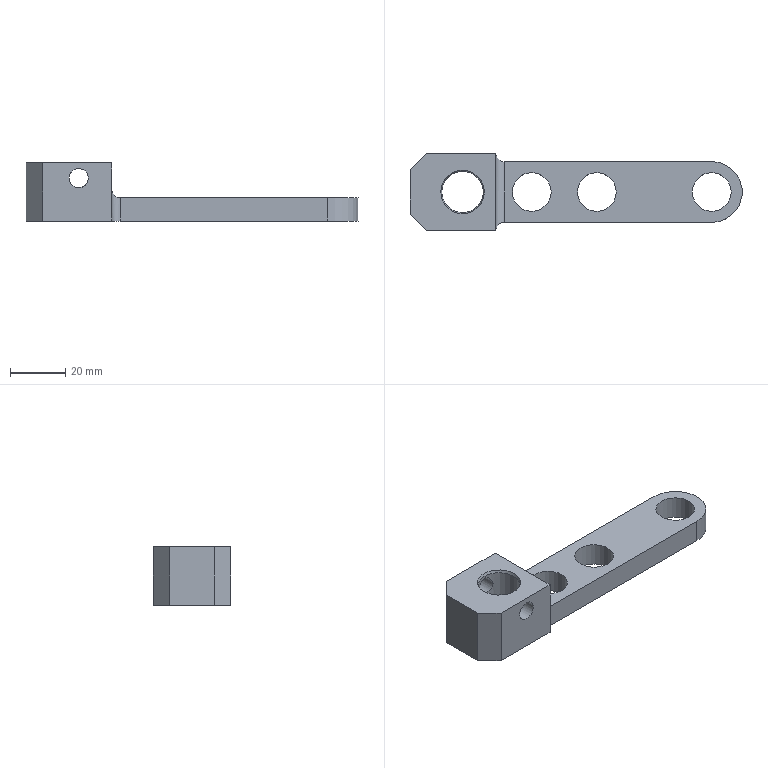NC program | NX | posted with a generic post | part box 120 x 28 x 21 mm
Lines 1 to 817 of 4754:
N10 G17 G21 G94 G90
(动态粗_COPY , TOOL : D10-30-D10-75-3T-粗)
N12 T02 M6
N14 G54
N16 G17 G0 G90 X10.538 Y8.528 B0. C0. S4500 M3
N18 G43 Z6. H2
N20 Z-11.9
N22 G94 G1 X10.513 Y8.53 Z-12.056 F2000.
N24 X10.488 Y8.531 Z-12.118
N26 X10.463 Y8.533 Z-12.163
N28 X10.438 Y8.534 Z-12.2
N30 X10.413 Y8.535 Z-12.231
N32 X10.388 Y8.537 Z-12.257
N34 X10.363 Y8.538 Z-12.28
N36 X10.338 Y8.54 Z-12.3
N38 X10.313 Y8.541 Z-12.318
N40 X10.288 Y8.543 Z-12.333
N42 X10.263 Y8.544 Z-12.347
N44 X10.238 Y8.545 Z-12.358
N46 X10.213 Y8.547 Z-12.368
N48 X10.188 Y8.548 Z-12.377
N50 X10.163 Y8.55 Z-12.384
N52 X10.138 Y8.551 Z-12.39
N54 X10.113 Y8.553 Z-12.394
N56 X10.089 Y8.554 Z-12.397
N58 X10.064 Y8.555 Z-12.399
N60 X10.039 Y8.557 Z-12.4
N62 X8.546 Y8.643
N64 G3 X7.508 Y7.879 R1.01
N66 X7.317 Y4.783 R18.753
N68 G1 X7.3 Y-0.166
N70 Y-13.665
N72 G2 X4.671 Y-18.222 R5.622
N74 X0.422 Y-19.616 R9.406
N76 X-4.852 Y-19.795 R53.755
N78 G1 X-8.512 Y-19.8
N80 X-121.12 Y-19.799
N82 G2 X-125.704 Y-17.192 R5.608
N84 X-127.105 Y-12.993 R9.323
N86 X-127.296 Y-7.224 R56.034
N88 G1 X-127.299 Y-3.624
N90 Y13.704
N92 G2 X-124.635 Y18.242 R5.634
N94 X-120.462 Y19.609 R9.412
N96 X-114.738 Y19.797 R56.511
N98 G1 X-111.138 Y19.8
N100 X1.21 Y19.798
N102 G2 X5.737 Y17.142 R5.633
N104 X7.119 Y12.868 R9.502
N106 X7.172 Y6.565 R41.659
N108 G3 X7.1 Y-5.331 R443.864
N110 G2 X7.078 Y-12.81 R298.984
N112 X3.379 Y-18.221 R6.758
N114 X-1.172 Y-19.434 R11.824
N116 X-7.693 Y-19.597 R82.236
N118 G1 X-10.783 Y-19.599
N120 X-119.765
N122 G2 X-125.66 Y-15.986 R6.715
N124 X-126.925 Y-11.406 R11.612
N126 X-127.096 Y-5.396 R71.864
N128 G1 X-127.099 Y-1.766
N130 X-127.098 Y12.354
N132 G2 X-123.451 Y18.179 R6.723
N134 X-118.932 Y19.423 R11.634
N136 X-112.996 Y19.596 R69.91
N138 G1 X-109.366 Y19.599
N140 X-0.146 Y19.598
N142 G2 X5.679 Y15.951 R6.723
N144 X6.929 Y11.364 R11.709
N146 X6.968 Y6.558 R40.739
N148 G3 X6.9 Y-10.921 R915.071
N150 G2 X2.447 Y-18.104 R7.514
N152 X-2.314 Y-19.238 R13.605
N154 X-9.6 Y-19.397 R102.013
N156 G1 X-12.48 Y-19.399
N158 X-118.475
N160 G2 X-125.623 Y-14.9 R7.517
N162 X-126.749 Y-10.045 R13.888
N164 X-126.898 Y-2.278 R116.141
N166 G1 X-126.899 Y10.959
N168 G2 X-122.384 Y18.131 R7.522
N170 X-117.541 Y19.25 R13.919
N172 X-109.789 Y19.398 R115.93
N174 G1 X-1.526 Y19.399
N176 G2 X5.592 Y14.965 R7.506
N178 X6.734 Y9.828 R13.309
N180 X6.719 Y3.366 R144.577
N182 G1 X6.69 Y-10.546
N184 G2 X1.74 Y-17.922 R8.049
N186 X-3.287 Y-19.042 R15.039
N188 G3 X-6.001 Y-19.2 R88.888
N190 G1 X-32.286
N192 X-117.501 Y-19.199
N194 G2 X-122.346 Y-17.925 R8.557
N196 X-125.874 Y-13.031 R8.81
N198 X-126.615 Y-7.985 R19.932
N200 X-126.699 Y0.849 R258.101
N202 X-126.678 Y10.808 R535.414
N204 X-121.799 Y17.892 R8.025
N206 X-116.852 Y19.032 R14.764
N208 X-109.085 Y19.198 R108.819
N210 G1 X-106.61 Y19.199
N212 X-30.999 Y19.2
N214 X-3.999 Y19.199
N216 G2 X-0.795 Y19.09 R23.657
N218 X5.374 Y14.337 R8.002
N220 X6.478 Y9.341 R13.791
N222 X6.539 Y6.702 R110.831
N224 X6.478 Y-10.019 R924.614
N226 X1.199 Y-17.694 R8.493
N228 X-3.935 Y-18.828 R15.836
N230 G3 X-4.987 Y-19.1 R5.087
N232 G1 X-5.495 Y-19.15
N234 G3 X-4.159 Y-18.849 R4.499
N236 X-0.89 Y-18.218 R61.535
N238 X4.035 Y-15.414 R9.864
N240 X6.241 Y-10.163 R8.958
N242 X6.417 Y-4.084 R71.286
N244 X6.384 Y8.466 R628.675
N246 X5.486 Y13.538 R15.499
N248 X-1.451 Y18.9 R8.213
N250 X-4.909 Y19.083 R39.059
N252 G1 X-4.953 Y19.091
N254 G2 X-5.655 Y19.749 R1.001
N256 G1 X-6.115 Y21.688 Z-12.3
N258 X-6.221 Y22.12 F15000.
N260 X-6.309 Y22.556
N262 G2 X-4.953 Y23.575 R1.
N264 X-4.243 Y22.892 R1.061
N266 X-4.845 Y21.663 R1.
N268 G1 X-4.977 Y21.613
N270 X-6.311 Y21.105 Z-12.372 F2000.
N272 G3 X-6.736 Y20.745 Z-12.4 R1.007
N274 X-5.999 Y19.2 R1.
N276 G2 X-4.21 Y18.966 R20.925
N278 X-0.76 Y18.495 R23.84
N280 X5.245 Y12.996 R8.609
N282 X6.15 Y7.892 R16.45
N284 X6.219 Y0.033 R239.909
N286 X6.115 Y-8.824 R183.204
N288 X4.883 Y-13.497 R10.616
N290 X-0.132 Y-17.601 R9.314
N292 X-3.382 Y-18.481 R27.849
N294 X-4.169 Y-18.852 R5.534
N296 G3 X-3.343 Y-18.458 R5.409
N298 X-0.477 Y-17.559 R99.779
N300 X4.494 Y-13.625 R9.518
N302 X5.925 Y-8.897 R10.992
N304 X6.098 Y-2.152 R77.601
N306 X6.076 Y6.471 R397.958
N308 X5.516 Y11.514 R22.957
N310 X2.216 Y16.758 R9.331
N312 X-2.325 Y18.573 R9.963
N314 G1 X-4.138 Y18.843
N316 X-4.899 Y19.074
N318 G3 X-1.738 Y18.244 R39.019
N320 G2 X5.042 Y11.819 R9.338
N322 X5.833 Y6.659 R19.711
N324 X5.882 Y-5.823 R379.658
N326 X5.414 Y-10.411 R23.249
N328 X2.946 Y-14.93 R9.333
N330 G1 X0.662 Y-17.214
N332 G3 X0.398 Y-17.632 R1.364
N334 G1 X-0.474 Y-19.425 Z-12.3
N336 X-0.877 Y-20.254 F15000.
N338 G3 X-0.498 Y-21.545 R1.
N340 G1 X-0.325 Y-21.652
N342 X-0.157 Y-21.767
N344 G2 X-1.625 Y-23.1 R-1.
N346 G1 X-3.007 Y-21.106
N348 X-3.428 Y-20.503 Z-12.337 F2000.
N350 X-3.841 Y-19.894 Z-12.374
N352 G2 X-3.982 Y-19.399 Z-12.4 R1.006
N354 X-3.453 Y-18.506 R1.001
N356 X-1.328 Y-17.721 R17.488
N358 G3 X2.166 Y-15.45 R10.608
N360 X5.455 Y-9.118 R10.513
N362 X5.772 Y-3.762 R35.277
N364 G1 X5.776 Y5.708
N366 G3 X5.219 Y10.523 R28.532
N368 X2.161 Y15.934 R10.113
N370 X-2.26 Y18.187 R10.905
N372 G1 X-3.586 Y18.577
N374 X-4.009 Y18.803
N376 G3 X-1.79 Y17.856 R13.22
N378 G2 X3.157 Y14.241 R10.391
N380 X5.216 Y8.889 R12.348
N382 X5.566 Y3.386 R34.911
N384 G1 X5.576 Y-5.364
N386 G2 X4.966 Y-10.108 R22.895
N388 X-1.622 Y-17.474 R11.081
N390 G3 X-2.686 Y-17.975 R8.519
N392 G2 X-3.337 Y-18.444 R2.537
N394 G3 X-2.551 Y-17.876 R4.482
N396 X-0.072 Y-16.514 R63.751
N398 X4.792 Y-10.014 R11.367
N400 X5.256 Y-7.797 R7.281
N402 X5.455 Y-2.389 R48.803
N404 G1 X5.453 Y5.731
N406 X5.083 Y9.117
N408 G3 X3.251 Y13.723 R13.39
N410 X2.079 Y15.16 R11.052
N412 G1 X0.283 Y16.956
N414 G2 X0.031 Y17.38 R1.021
N416 X1.124 Y18.654 Z-12.3 R1.002
N418 G1 X1.269 Y18.622 F15000.
N420 X1.408 Y18.571
N422 X4.478 Y17.157
N424 X4.63 Y17.068
N426 X4.767 Y16.956
N428 X6.388 Y15.335
N430 G2 X7.344 Y13.237 R3.292
N432 G1 X7.43 Y12.01
N434 G2 X7.238 Y11.348 R1.005
N436 G1 X7.05 Y11.093
N438 X5.87 Y9.488 Z-12.4 F2000.
N440 X5.577 Y9.096
N442 X5.299 Y8.693
N444 G3 X5.188 Y8.127 R1.011
N446 G2 X5.253 Y-5.397 R549.731
N448 G3 X5.2 Y-8.001 R25.182
N450 G1 X5.1 Y-9.016
N452 X5.2 Y-8.001
N454 Y8.
N456 G3 X4.805 Y9.989 R6.055
N458 X2.673 Y14.158 R13.609
N460 X-2.022 Y17.747 R10.723
N462 G2 X-2.917 Y18.166 R11.664
N464 X-3.311 Y19.015 R1.001
N466 X-3.166 Y19.519 Z-12.374 R1.504
N468 G1 X-2.616 Y20.877 Z-12.3
N470 X-2.284 Y21.694 F15000.
N472 G2 X-0.675 Y22.049 R1.
N474 G1 X-0.415 Y21.809
N476 X-0.166 Y21.558
N478 G2 X-1.164 Y19.962 R1.
N480 G1 X-2.789 Y20.363 Z-12.384 F2000.
N482 X-2.947 Y20.379 Z-12.392
N484 X-3.106 Y20.372 Z-12.4
N486 G3 X-3.441 Y18.5 R1.
N488 G2 X-2.679 Y17.994 R4.582
N490 X-0.143 Y16.462 R31.336
N492 X3.992 Y11.3 R12.947
N494 G1 X4.324 Y10.888
N496 X4.805 Y9.989
N498 X4.324 Y10.888
N500 G2 X3.286 Y12.426 R9.707
N502 G3 X-1.647 Y17.218 R13.806
N504 G2 X-2.856 Y18.114 R6.817
N506 G3 X-0.329 Y16.083 R47.298
N508 G2 X3.085 Y12.269 R17.62
N510 X4.001 Y11.282 R8.895
N512 G3 X2.855 Y12.519 R18.595
N514 X-1.364 Y16.718 R23.285
N516 G1 X-2.181 Y17.535
N518 X3.037 Y12.317
N520 G3 X4.059 Y12.074 R1.001
N522 G1 X4.521 Y12.288 Z-12.374
N524 X4.975 Y12.516 Z-12.349
N526 X5.85 Y12.948 Z-12.3
N528 X6.224 Y13.12 F15000.
N530 G2 X7.521 Y12.317 R1.
N532 G1 X7.78 Y10.595
N534 X8.023 Y8.871
N536 G2 X8.324 Y4.909 R41.634
N538 G1 X8.675 Y-7.772
N540 G2 X7.962 Y-8.757 R1.
N542 G1 X7.636 Y-8.855
N544 X5.727 Y-9.425 Z-12.4 F2000.
N546 X5.264 Y-9.573
N548 G3 X4.792 Y-10.014 R1.007
N550 G2 X3.206 Y-12.877 R26.269
N552 X1.795 Y-14.584 R13.407
N554 X0.165 Y-16.183 R33.637
N556 G3 X-2.035 Y-17.397 R184.505
N558 G2 X-2.66 Y-17.953 R17.962
N560 G1 X-1.894 Y-17.28
N562 G3 X1.034 Y-15.102 R17.88
N564 X3.9 Y-11.405 R14.788
N566 X4.641 Y-10.295 R3.607
N568 G2 X3.9 Y-11.405 R3.607
N570 X1.494 Y-14.278 R38.395
N572 X-1.136 Y-16.489 R19.494
N574 G1 X-2.069 Y-17.423
N576 G2 X0.512 Y-15.025 R38.919
N578 G3 X2.884 Y-12.47 R20.143
N580 G1 X3.676 Y-11.677
N582 X-1.051 Y-16.405
N584 G3 X-1.247 Y-17.553 R1.028
N586 G1 X-0.548 Y-19.419 Z-12.3
N588 G2 X-0.417 Y-19.882 R1.544 F15000.
N590 X-1.051 Y-20.889 R1.
N592 G1 X-3.171 Y-21.707
N594 X-3.712 Y-21.886
N596 X-4.262 Y-22.035
N598 G2 X-5.183 Y-22.138 R4.839
N600 G1 X-27.83 Y-22.371
N602 G2 X-28.662 Y-21.941 R1.001
N604 G1 X-28.826 Y-21.704
N606 X-29.963 Y-20.067 Z-12.4 F2000.
N608 X-30.154 Y-19.785
N610 X-30.36 Y-19.512
N612 G3 X-31.001 Y-19.2 R1.005
N614 X-36.128 Y-19.005 R47.114
N616 G1 X-39.411 Y-19.
N618 X-116.376 Y-18.999
N620 G2 X-120.417 Y-18.405 R10.948
N622 X-125.31 Y-13.419 R8.626
N624 X-126.355 Y-8.218 R16.886
N626 X-126.497 Y-0.271 R134.652
N628 X-126.477 Y9.984 R692.384
N630 X-121.233 Y17.677 R8.488
N632 X-116.102 Y18.826 R15.741
N634 X-108.921 Y18.996 R101.92
N636 G1 X-105.996 Y18.999
N638 X-32.471
N640 X-32.248 Y19.029
N642 G3 X-31.523 Y19.872 R1.001
N644 X-31.815 Y20.713 Z-12.354 R1.047
N646 G1 X-32.508 Y21.532 Z-12.3
N648 X-32.708 Y21.765 F15000.
N650 X-32.896 Y22.008
N652 G2 X-32.248 Y23.513 R1.
N654 X-31.019 Y22.895 R1.017
N656 G1 X-30.588 Y21.714
N658 X-30.139 Y20.467 Z-12.367 F2000.
N660 G2 X-30.174 Y19.814 Z-12.4 R1.001
N662 X-31.001 Y19.2 R1.001
N664 G3 X-32.503 Y18.98 R7.645
N666 G2 X-37.235 Y18.879 R58.27
N668 G1 X-105.101
N670 G3 X-114.945 Y18.769 R223.
N672 X-120.178 Y17.885 R18.893
N674 X-125.26 Y13.641 R8.822
N676 X-126.311 Y9.224 R10.712
N678 X-126.378 Y0.735 R217.59
N680 X-126.243 Y-7.888 R155.516
N682 X-125.246 Y-13.052 R17.247
N684 X-117.982 Y-18.7 R8.632
N686 X-112.933 Y-18.877 R44.096
N688 G1 X-110.458 Y-18.879
N690 X-38.673 Y-18.88
N692 G2 X-32.423 Y-18.983 R96.355
N694 G1 X-31.928 Y-19.116
N696 G3 X-34.626 Y-18.74 R9.534
N698 X-41.736 Y-18.68 R280.612
N700 G1 X-111.471 Y-18.679
N702 G2 X-117.047 Y-18.549 R65.812
N704 X-122.611 Y-16.199 R9.255
N706 X-125.511 Y-10.962 R10.343
N708 X-126.116 Y-5.515 R26.74
N710 X-126.123 Y8.494 R342.264
N712 X-125.141 Y12.991 R11.374
N714 X-119.957 Y17.554 R9.129
N716 X-114.608 Y18.544 R18.512
N718 X-105.325 Y18.678 R175.862
N720 G1 X-39.476
N722 G3 X-33.186 Y18.761 R107.31
N724 G1 X-32.982 Y18.807
N726 G3 X-32.463 Y19.534 R1.002
N728 G1 X-32.454 Y19.791 Z-12.387
N730 X-32.471 Y20.048 Z-12.374
N732 X-32.565 Y21.523 Z-12.3
N734 X-32.617 Y22.352 F15000.
N736 G3 X-34.142 Y23.138 R1.
N738 G1 X-34.396 Y22.983
N740 X-34.641 Y22.816
N742 G3 X-34.074 Y21.056 R1.
N744 G1 X-32.445 Y20.967 Z-12.382 F2000.
N746 X-32.269 Y20.929 Z-12.391
N748 X-32.102 Y20.861 Z-12.4
N750 G2 X-32.28 Y19.019 R1.
N752 X-34.916 Y18.6 R7.682
N754 X-40.081 Y18.558 R547.93
N756 G1 X-105.686
N758 G3 X-114.549 Y18.415 R155.99
N760 X-119.818 Y17.405 R17.982
N762 X-125.754 Y10.111 R9.141
N764 X-126.049 Y5.356 R30.278
N766 X-125.96 Y-6.238 R287.079
N768 X-125.153 Y-11.608 R21.292
N770 X-121.272 Y-16.896 R9.444
N772 X-116.344 Y-18.419 R10.827
N774 X-110.017 Y-18.559 R80.121
N776 G1 X-42.315 Y-18.56
N778 G2 X-34.139 Y-18.659 R162.972
N780 X-32.943 Y-18.815 R6.107
N782 X-33.623 Y-20.695 R1.
N784 G1 X-33.808 Y-20.635
N786 X-34.701 Y-20.339 Z-12.353
N788 X-35.599 Y-20.057 Z-12.306
N790 X-35.709 Y-20.04 Z-12.3
N792 G3 X-36.113 Y-21.986 R1. F15000.
N794 G1 X-35.838 Y-22.079
N796 X-35.559 Y-22.156
N798 G3 X-34.96 Y-22.069 R1.009
N800 G1 X-33.403 Y-21.314
N802 X-32.306 Y-20.777 Z-12.361 F2000.
N804 G3 X-31.841 Y-20.187 Z-12.4 R1.
N806 X-32.537 Y-18.948 R1.
N808 G1 X-33.361 Y-18.678
N810 G3 X-37.088 Y-18.391 R21.163
N812 G1 X-43.236 Y-18.36
N814 X-109.496 Y-18.359
N816 G2 X-115.898 Y-18.22 R81.598
N818 X-120.892 Y-16.667 R10.913
N820 X-124.87 Y-11.312 R9.799
N822 X-125.741 Y-5.893 R21.049
N824 X-125.786 Y7.455 R215.609
N826 X-124.859 Y12.078 R13.328
N828 X-119.309 Y17.195 R9.445
N830 X-113.843 Y18.215 R19.034
N832 X-105.82 Y18.357 R144.795
N834 G1 X-102.85 Y18.359
N836 X-39.78
N838 G3 X-34.168 Y18.472 R74.504
N840 X-33.288 Y18.644 R3.293
N842 X-32.849 Y19.108 R1.007
N844 G1 X-32.519 Y19.824
N846 X-31.684 Y21.634 Z-12.3
N848 X-31.558 Y21.908 F15000.
N850 X-31.423 Y22.178
N852 G2 X-31.046 Y22.528 R1.017
N854 G1 X-30.823 Y22.647
N856 X-30.594 Y22.754
N858 G2 X-29.272 Y21.705 R1.
N860 X-29.79 Y20.925 Z-12.349 R1.041 F2000.
N862 G1 X-30.639 Y20.36 Z-12.4
N864 X-32.891 Y18.86
N866 G2 X-34.5 Y18.378 R3.258
N868 X-40.236 Y18.24 R68.313
N870 G1 X-42.211 Y18.238
N872 X-104.826
N874 G3 X-113.703 Y18.091 R157.127
N876 X-119.109 Y17.073 R18.827
N878 X-125.336 Y9.675 R9.575
N880 X-125.722 Y4.642 R27.891
N882 X-125.61 Y-5.886 R193.965
N884 X-124.667 Y-11.353 R19.978
N886 X-117.196 Y-17.832 R9.588
N888 X-112.148 Y-18.223 R27.745
N890 G1 X-107.258 Y-18.239
N892 X-42.468 Y-18.24
N894 G2 X-35.012 Y-18.367 R120.469
N896 X-33.306 Y-18.638 R7.99
N898 G1 X-32.982 Y-18.794
N900 G3 X-35.053 Y-18.237 R5.187
N902 X-40.824 Y-18.046 R62.867
N904 G1 X-44.826 Y-18.04
N906 X-108.081 Y-18.039
N908 G2 X-114.887 Y-17.896 R91.661
N910 X-119.927 Y-16.506 R12.305
N912 X-124.445 Y-10.905 R9.972
N914 X-125.399 Y-5.409 R20.561
N916 X-125.437 Y6.827 R147.617
N918 X-124.361 Y11.721 R13.762
N920 X-118.584 Y16.882 R9.838
N922 X-113.157 Y17.883 R19.706
N924 X-103.89 Y18.038 R161.28
N926 G1 X-43.196
N928 G3 X-35.45 Y18.131 R154.121
N930 X-33.754 Y18.397 R5.986
N932 G1 X-33.317 Y18.629
N934 G2 X-35.206 Y18.076 R4.016
N936 X-40.944 Y17.92 R65.872
N938 G1 X-42.917 Y17.918
N940 X-103.576
N942 G3 X-112.769 Y17.776 R173.328
N944 X-118.276 Y16.801 R20.239
N946 X-124.924 Y9.264 R9.955
N948 X-125.391 Y4.149 R25.916
N950 X-125.253 Y-5.613 R136.872
N952 X-124.181 Y-11.099 R18.919
N954 X-116.744 Y-17.43 R9.942
N956 X-111.598 Y-17.894 R26.267
N958 G1 X-105.868 Y-17.919
N960 X-43.429 Y-17.92
N962 G2 X-35.832 Y-18.064 R116.313
N964 X-33.737 Y-18.424 R7.724
N966 G1 X-33.711 Y-18.438
N968 G2 X-34.143 Y-20.298 R1.
N970 X-34.691 Y-20.201 Z-12.372 R1.417
N972 G1 X-36.061 Y-19.783 Z-12.3
N974 G3 X-37.431 Y-20.632 R1.011 F15000.
N976 X-36.881 Y-21.609 R1.001
N978 G1 X-36.676 Y-21.711
N980 X-36.466 Y-21.805
N982 G3 X-35.637 Y-21.713 R1.002
N984 G1 X-34.339 Y-20.934
N986 X-33.289 Y-20.298 Z-12.362 F2000.
N988 G3 X-32.88 Y-19.674 Z-12.4 R1.001
N990 X-33.428 Y-18.579 R1.
N992 X-35.536 Y-17.962 R5.08
N994 X-41.328 Y-17.729 R54.775
N996 G1 X-46.056 Y-17.72
N998 X-106.746 Y-17.719
N1000 G2 X-113.883 Y-17.581 R105.451
N1002 X-119.034 Y-16.302 R13.708
N1004 X-124.076 Y-10.366 R10.228
N1006 X-125.074 Y-4.666 R21.056
N1008 X-125.09 Y6.249 R109.89
N1010 X-123.907 Y11.318 R14.116
N1012 X-117.944 Y16.548 R10.184
N1014 X-112.308 Y17.565 R20.611
N1016 X-103.49 Y17.717 R158.554
N1018 G1 X-100.52 Y17.718
N1020 X-42.555 Y17.719
N1022 G3 X-35.85 Y17.849 R96.535
N1024 X-34.08 Y18.186 R5.686
N1026 G1 X-34.003 Y18.233
N1028 G3 X-33.57 Y18.958 R1.002
N1030 G1 X-33.533 Y19.32
N1032 X-33.329 Y21.302 Z-12.3
N1034 X-33.297 Y21.644 F15000.
N1036 X-33.248 Y21.984
N1038 G2 X-32.843 Y22.564 R1.005
N1040 G1 X-32.506 Y22.781
N1042 G2 X-31.086 Y21.699 R1.
N1044 X-31.365 Y21.165 Z-12.331 R1.099 F2000.
N1046 G1 X-32.251 Y20.105 Z-12.4
N1048 X-33.495 Y18.618
N1050 G2 X-35.2 Y17.858 R2.823
N1052 X-39.856 Y17.611 R34.191
N1054 G1 X-44.401 Y17.598
N1056 X-102.236
N1058 G3 X-111.954 Y17.456 R189.211
N1060 X-117.612 Y16.478 R21.173
N1062 X-124.558 Y8.702 R10.317
N1064 X-125.063 Y3.44 R26.106
N1066 X-124.867 Y-5.629 R95.029
N1068 X-123.566 Y-11.152 R17.228
N1070 X-116.359 Y-17.022 R10.232
N1072 X-111.222 Y-17.561 R24.665
N1074 X-104.142 Y-17.599 R603.963
N1076 G1 X-44.928 Y-17.6
N1078 G2 X-36.713 Y-17.747 R131.63
N1080 X-34.011 Y-18.236 R9.341
N1082 G1 X-33.88 Y-18.309
N1084 G2 X-34.182 Y-20.089 R1.
N1086 X-34.802 Y-20.07 Z-12.368 R1.093
N1088 G1 X-36.122 Y-19.726 Z-12.3
N1090 G3 X-37.368 Y-20.243 R1.02 F15000.
N1092 X-37.051 Y-21.48 R1.
N1094 X-36.606 Y-21.752 R1.774
N1096 X-35.659 Y-21.599 R1.001
N1098 G1 X-34.627 Y-20.797
N1100 X-34.112 Y-20.401 Z-12.333 F2000.
N1102 X-33.605 Y-19.996 Z-12.365
N1104 G3 X-33.285 Y-19.397 Z-12.4 R1.001
N1106 X-33.688 Y-18.448 R1.001
N1108 X-35.346 Y-17.788 R3.523
N1110 X-40.06 Y-17.437 R30.027
N1112 X-47.271 Y-17.4 R612.258
N1114 G1 X-105.501 Y-17.399
N1116 G2 X-113.118 Y-17.253 R112.063
N1118 X-118.368 Y-15.992 R14.599
N1120 X-123.685 Y-9.918 R10.476
N1122 X-124.74 Y-4.107 R21.083
N1124 X-124.728 Y5.891 R81.568
N1126 X-123.321 Y11.208 R13.86
N1128 X-117.346 Y16.211 R10.525
N1130 X-111.666 Y17.236 R21.112
N1132 X-102.774 Y17.396 R155.096
N1134 G1 X-99.519 Y17.398
N1136 X-43.381 Y17.399
N1138 G3 X-36.511 Y17.54 R96.911
N1140 X-34.328 Y17.982 R6.773
N1142 G1 X-33.971 Y18.255
N1144 G2 X-35.312 Y17.638 R2.51
N1146 X-39.516 Y17.309 R24.209
N1148 G1 X-46.111 Y17.278
N1150 X-101.506 Y17.277
N1152 G3 X-111.179 Y17.135 R191.785
N1154 X-116.932 Y16.169 R22.182
N1156 X-124.179 Y8.239 R10.628
N1158 X-124.731 Y2.878 R25.583
N1160 X-124.483 Y-5.514 R71.59
N1162 X-122.956 Y-11.145 R16.23
N1164 X-115.897 Y-16.641 R10.524
N1166 X-110.421 Y-17.238 R25.19
N1168 X-102.936 Y-17.279 R612.727
N1170 G1 X-45.964 Y-17.28
N1172 G2 X-37.495 Y-17.43 R139.709
N1174 X-34.445 Y-17.962 R11.219
N1176 X-33.945 Y-18.262 R2.394
N1178 G3 X-35.72 Y-17.521 R3.826
N1180 X-40.47 Y-17.128 R28.676
N1182 X-48.351 Y-17.08 R618.379
N1184 G1 X-104.371 Y-17.079
N1186 G2 X-112.198 Y-16.941 R126.511
N1188 X-117.576 Y-15.752 R15.896
N1190 X-123.344 Y-9.357 R10.739
N1192 X-124.408 Y-3.533 R21.42
N1194 X-124.36 Y5.579 R62.896
N1196 X-122.764 Y11.039 R13.684
N1198 X-116.723 Y15.891 R10.856
N1200 X-110.905 Y16.917 R21.985
N1202 X-101.278 Y17.077 R173.638
N1204 G1 X-46.451 Y17.078
N1206 G3 X-37.77 Y17.184 R181.979
N1208 X-34.851 Y17.642 R11.258
N1210 X-34.23 Y18.044 R1.853
N1212 G2 X-35.753 Y17.347 R2.865
N1214 X-40.223 Y16.991 R25.69
N1216 G1 X-46.606 Y16.958
N1218 X-100.641 Y16.957
N1220 G3 X-110.569 Y16.807 R191.107
N1222 X-116.38 Y15.826 R22.63
N1224 X-122.78 Y10.539 R10.889
N1226 X-124.252 Y5.037 R14.72
N1228 X-124.076 Y-5.521 R55.893
N1230 X-122.278 Y-11.222 R15.247
N1232 X-115.389 Y-16.281 R10.82
N1234 X-109.781 Y-16.912 R25.523
N1236 X-101.691 Y-16.96 R574.396
N1238 G1 X-47.133
N1240 G2 X-38.311 Y-17.107 R155.983
N1242 X-34.901 Y-17.67 R13.107
N1244 X-34.435 Y-17.903 R2.799
N1246 X-35.535 Y-19.547 R1.
N1248 G1 X-36.04 Y-19.238 Z-12.37
N1250 X-36.536 Y-18.915 Z-12.341
N1252 X-37.218 Y-18.479 Z-12.3
N1254 G3 X-38.318 Y-20.145 R1. F15000.
N1256 X-37.903 Y-20.403 R1.531
N1258 X-37.332 Y-20.437 R1.011
N1260 G1 X-35.741 Y-20.066
N1262 X-34.565 Y-19.786 Z-12.361 F2000.
N1264 G3 X-33.976 Y-19.301 Z-12.4 R1.
N1266 X-34.273 Y-18.024 R1.
N1268 X-35.957 Y-17.277 R3.644
N1270 X-40.497 Y-16.83 R25.169
N1272 X-49.536 Y-16.76 R384.859
N1274 G1 X-103.321 Y-16.759
N1276 G2 X-111.478 Y-16.617 R133.57
N1278 X-116.883 Y-15.471 R16.814
N1280 X-122.997 Y-8.832 R10.991
N1282 X-124.082 Y-2.859 R21.892
N1284 X-123.966 Y5.455 R48.744
N1286 X-122.058 Y11.106 R13.211
N1288 X-115.936 Y15.633 R11.268
N1290 X-109.927 Y16.613 R23.776
N1292 X-100.239 Y16.757 R196.493
N1294 G1 X-47.726 Y16.758
N1296 G3 X-38.469 Y16.865 R201.933
N1298 X-35.247 Y17.356 R12.721
N1300 X-34.717 Y17.636 R1.701
N1302 X-34.419 Y18.195 R1.008
N1304 G1 X-34.259 Y19.144
N1306 X-33.928 Y21.109 Z-12.3
N1308 X-33.85 Y21.515 F15000.
N1310 G2 X-33.557 Y21.967 R1.014
N1312 X-33.123 Y22.285 R1.671
N1314 X-31.761 Y21.644 R1.
N1316 X-32.035 Y20.636 Z-12.355 R1.036 F2000.
N1318 G1 X-32.625 Y19.961 Z-12.4
N1320 X-34.481 Y17.844
N1322 G2 X-36.369 Y17.015 R3.597
N1324 X-41.257 Y16.666 R30.754
N1326 G1 X-48.106 Y16.638
N1328 X-99.816 Y16.637
N1330 G3 X-109.908 Y16.483 R193.672
N1332 X-115.866 Y15.477 R23.15
N1334 X-122.368 Y10.142 R11.142
N1336 X-123.902 Y4.566 R14.854
N1338 X-123.655 Y-5.535 R45.273
N1340 X-121.565 Y-11.305 R14.488
N1342 X-114.79 Y-15.95 R11.145
N1344 X-109.197 Y-16.586 R26.116
N1346 X-100.487 Y-16.64 R479.165
N1348 G1 X-48.677
N1350 G2 X-39.154 Y-16.779 R184.214
N1352 X-35.399 Y-17.355 R15.401
N1354 X-34.562 Y-17.773 R2.755
N1356 X-35.536 Y-19.453 R1.
N1358 G1 X-35.75 Y-19.361 Z-12.388
N1360 X-35.949 Y-19.24 Z-12.377
N1362 X-37.247 Y-18.438 Z-12.3
N1364 G3 X-38.445 Y-20.015 R1. F15000.
N1366 X-37.962 Y-20.38 R1.353
N1368 X-37.277 Y-20.395 R1.005
N1370 G1 X-35.923 Y-19.933
N1372 X-34.754 Y-19.53 Z-12.362 F2000.
N1374 G3 X-34.226 Y-19.015 Z-12.4 R1.001
N1376 X-34.427 Y-17.909 R1.001
N1378 X-35.815 Y-17.134 R2.81
N1380 X-39.979 Y-16.562 R18.389
N1382 X-50.676 Y-16.44 R246.684
N1384 G1 X-102.471 Y-16.439
N1386 G2 X-110.779 Y-16.295 R137.644
N1388 X-116.334 Y-15.137 R17.511
N1390 X-122.644 Y-8.343 R11.222
N1392 X-123.746 Y-2.328 R21.969
N1394 X-123.554 Y5.397 R38.79
N1396 X-121.201 Y11.335 R12.723
N1398 X-115.119 Y15.384 R11.761
N1400 X-109.023 Y16.304 R25.666
N1402 X-99.605 Y16.437 R210.529
N1404 G1 X-97.04 Y16.438
N1406 X-46.814
N1408 G3 X-38.633 Y16.577 R138.384
N1410 X-35.438 Y17.145 R11.267
N1412 X-34.807 Y17.518 R1.89
N1414 X-34.566 Y17.99 R1.015
N1416 G1 X-34.324 Y19.161
N1418 X-33.921 Y21.113 Z-12.3
N1420 X-33.827 Y21.528 F15000.
N1422 X-33.751 Y21.696
N1424 X-33.647 Y21.849
N1426 G2 X-33.281 Y22.22 R1.734
N1428 X-31.765 Y21.641 R1.
N1430 X-32.043 Y20.653 Z-12.354 R1.032 F2000.
N1432 G1 X-32.651 Y19.966 Z-12.4
N1434 X-34.638 Y17.719
N1436 G2 X-35.836 Y16.955 R2.147
N1438 X-39.506 Y16.425 R15.041
N1440 X-49.471 Y16.318 R233.054
N1442 G1 X-99.051 Y16.317
N1444 G3 X-109.218 Y16.163 R198.156
N1446 X-115.213 Y15.18 R24.122
N1448 X-121.592 Y10.386 R11.492
N1450 X-123.49 Y4.631 R13.94
N1452 X-123.211 Y-5.607 R37.187
N1454 X-120.719 Y-11.521 R13.754
N1456 X-114.123 Y-15.642 R11.529
N1458 X-108.392 Y-16.267 R27.745
N1460 X-99.053 Y-16.32 R539.024
N1462 G1 X-49.652
N1464 G2 X-39.685 Y-16.469 R187.585
N1466 X-35.768 Y-17.073 R16.376
N1468 X-34.615 Y-17.718 R2.498
N1470 G3 X-36.085 Y-16.876 R3.038
N1472 X-40.156 Y-16.269 R17.78
N1474 X-48.834 Y-16.121 R166.842
N1476 G1 X-97.886 Y-16.12
N1478 G2 X-109.035 Y-16.032 R332.376
N1480 X-114.717 Y-15.192 R22.422
N1482 X-122.309 Y-7.82 R11.467
N1484 X-123.421 Y-1.548 R22.374
N1486 X-123.108 Y5.465 R31.06
N1488 X-120.157 Y11.696 R12.249
N1490 X-114.168 Y15.171 R12.44
N1492 X-107.89 Y16.005 R28.783
N1494 X-96.176 Y16.118 R321.704
N1496 G1 X-47.638
N1498 G3 X-39.237 Y16.259 R146.099
N1500 X-35.76 Y16.859 R12.735
N1502 X-34.805 Y17.519 R1.83
N1504 G2 X-35.989 Y16.727 R2.207
N1506 X-39.713 Y16.129 R14.339
N1508 X-48.272 Y15.998 R165.604
N1510 G1 X-95.571
N1512 G3 X-107.595 Y15.89 R349.431
N1514 X-113.891 Y15.08 R29.447
N1516 X-120.005 Y11.545 R12.446
N1518 X-122.957 Y5.308 R12.447
N1520 X-123.212 Y-2.556 R30.619
N1522 X-121.787 Y-8.653 R18.869
N1524 X-113.955 Y-15.213 R11.534
N1526 X-108.222 Y-15.929 R25.804
N1528 X-98.086 Y-16. R385.467
N1530 G1 X-49.908
N1532 G2 X-40.132 Y-16.161 R174.629
N1534 X-36.041 Y-16.813 R16.724
N1536 X-34.977 Y-17.35 R3.416
N1538 X-35.691 Y-18.928 R1.
N1540 X-36.37 Y-18.753 Z-12.364 R1.081
N1542 G1 X-37.481 Y-18.12 Z-12.3
N1544 G3 X-37.932 Y-17.915 R1.486 F15000.
N1546 X-38.86 Y-19.592 R1.
N1548 X-38.487 Y-19.917 R1.702
N1550 X-37.671 Y-19.992 R1.002
N1552 G1 X-36.353 Y-19.541
N1554 X-35.154 Y-19.126 Z-12.364 F2000.
N1556 G3 X-34.639 Y-18.641 Z-12.4 R1.001
N1558 X-34.826 Y-17.504 R1.
N1560 X-36.298 Y-16.631 R3.082
N1562 X-40.453 Y-15.97 R17.391
N1564 X-50.198 Y-15.801 R169.834
N1566 G1 X-96.786 Y-15.8
N1568 G2 X-108.245 Y-15.716 R366.469
N1570 X-114.054 Y-14.9 R23.835
N1572 X-121.986 Y-7.277 R11.693
N1574 X-123.08 Y-0.807 R22.439
N1576 X-122.546 Y5.946 R24.64
N1578 X-114.782 Y14.486 R11.694
N1580 X-108.586 Y15.609 R23.377
N1582 X-99.425 Y15.794 R153.151
N1584 G1 X-95.21 Y15.798
N1586 X-48.463
N1588 G3 X-39.694 Y15.948 R148.255
N1590 X-36.037 Y16.584 R13.56
N1592 X-34.99 Y17.295 R1.995
N1594 G2 X-36.187 Y16.478 R2.285
N1596 X-39.905 Y15.834 R14.043
N1598 X-48.378 Y15.678 R141.27
N1600 G1 X-95.241 Y15.677
N1602 G3 X-107.224 Y15.557 R314.765
N1604 X-113.572 Y14.693 R28.757
N1606 X-119.786 Y10.949 R12.5
N1608 X-122.638 Y4.63 R12.786
N1610 X-122.227 Y-5.928 R26.823
N1612 X-118.592 Y-12.165 R12.589
N1614 X-112.381 Y-15.123 R12.786
N1616 X-106.321 Y-15.641 R35.11
N1618 X-96.771 Y-15.68 R686.715
N1620 G1 X-50.823
N1622 G2 X-40.752 Y-15.841 R185.4
N1624 X-36.486 Y-16.49 R18.554
N1626 X-35.075 Y-17.221 R3.5
N1628 G1 X-35.046 Y-17.256
N1630 G2 X-35.672 Y-18.86 R1.
N1632 X-36.393 Y-18.707 Z-12.362 R1.064